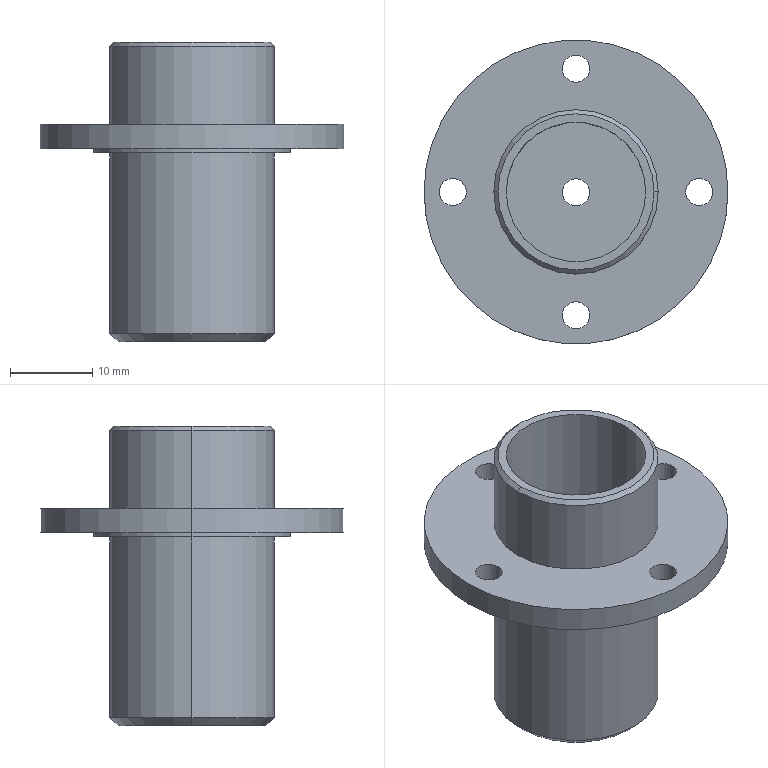Part | SolidWorks | features ICE 4, Chamfer 2, HoleWzd 2, 3DProfileFeature 1, Extrusion 1 | 1 solid | 30 faces | box 37 x 37 x 36.5 mm | volume 6267 mm3 | cylinder 20 | plane 6 | cone 4 | commonest cylinder face diameters 3.3 x10 20 x4 17 x2 24 x2 37 x2
STEP:
#1=CARTESIAN_POINT('',(9.5,0.,10.));
#2=VERTEX_POINT('',#1);
#3=CARTESIAN_POINT('',(-9.5,0.,10.));
#4=VERTEX_POINT('',#3);
#5=CARTESIAN_POINT('',(0.,0.,10.));
#6=DIRECTION('',(0.,0.,1.));
#7=DIRECTION('',(1.,0.,0.));
#8=AXIS2_PLACEMENT_3D('',#5,#6,#7);
#9=CIRCLE('',#8,9.5);
#10=EDGE_CURVE('',#2,#4,#9,.T.);
#11=ORIENTED_EDGE('',*,*,#10,.F.);
#12=CARTESIAN_POINT('',(10.,0.,9.5));
#13=VERTEX_POINT('',#12);
#14=CARTESIAN_POINT('',(9.5,0.,10.));
#15=DIRECTION('',(0.7071,0.,-0.7071));
#16=VECTOR('',#15,1000.);
#17=LINE('',#14,#16);
#18=EDGE_CURVE('',#2,#13,#17,.T.);
#19=ORIENTED_EDGE('',*,*,#18,.T.);
#20=CARTESIAN_POINT('',(-10.,0.,9.5));
#21=VERTEX_POINT('',#20);
#22=CARTESIAN_POINT('',(0.,0.,9.5));
#23=DIRECTION('',(0.,0.,-1.));
#24=DIRECTION('',(1.,0.,0.));
#25=AXIS2_PLACEMENT_3D('',#22,#23,#24);
#26=CIRCLE('',#25,10.);
#27=EDGE_CURVE('',#21,#13,#26,.T.);
#28=ORIENTED_EDGE('',*,*,#27,.F.);
#29=CARTESIAN_POINT('',(-9.5,0.,10.));
#30=DIRECTION('',(-0.7071,0.,-0.7071));
#31=VECTOR('',#30,1000.);
#32=LINE('',#29,#31);
#33=EDGE_CURVE('',#4,#21,#32,.T.);
#34=ORIENTED_EDGE('',*,*,#33,.F.);
#35=EDGE_LOOP('',(#11,#19,#28,#34));
#36=FACE_OUTER_BOUND('',#35,.T.);
#37=CARTESIAN_POINT('',(0.,0.,10.));
#38=DIRECTION('',(0.,0.,-1.));
#39=DIRECTION('',(-1.,0.,0.));
#40=AXIS2_PLACEMENT_3D('',#37,#38,#39);
#41=CONICAL_SURFACE('',#40,9.5,0.7854);
#42=ADVANCED_FACE('',(#36),#41,.T.);
#43=CARTESIAN_POINT('',(1.65,0.,-22.5));
#44=VERTEX_POINT('',#43);
#45=CARTESIAN_POINT('',(-1.65,0.,-22.5));
#46=VERTEX_POINT('',#45);
#47=CARTESIAN_POINT('',(0.,0.,-22.5));
#48=DIRECTION('',(0.,0.,-1.));
#49=DIRECTION('',(-1.,0.,0.));
#50=AXIS2_PLACEMENT_3D('',#47,#48,#49);
#51=CIRCLE('',#50,1.65);
#52=EDGE_CURVE('',#44,#46,#51,.T.);
#53=ORIENTED_EDGE('',*,*,#52,.F.);
#54=CARTESIAN_POINT('',(1.65,0.,-26.5));
#55=VERTEX_POINT('',#54);
#56=CARTESIAN_POINT('',(1.65,0.,-26.5));
#57=DIRECTION('',(0.,0.,-1.));
#58=VECTOR('',#57,1000.);
#59=LINE('',#56,#58);
#60=EDGE_CURVE('',#44,#55,#59,.T.);
#61=ORIENTED_EDGE('',*,*,#60,.T.);
#62=CARTESIAN_POINT('',(-1.65,0.,-26.5));
#63=VERTEX_POINT('',#62);
#64=CARTESIAN_POINT('',(0.,0.,-26.5));
#65=DIRECTION('',(0.,0.,-1.));
#66=DIRECTION('',(-1.,0.,0.));
#67=AXIS2_PLACEMENT_3D('',#64,#65,#66);
#68=CIRCLE('',#67,1.65);
#69=EDGE_CURVE('',#55,#63,#68,.T.);
#70=ORIENTED_EDGE('',*,*,#69,.T.);
#71=CARTESIAN_POINT('',(-1.65,0.,-26.5));
#72=DIRECTION('',(0.,0.,-1.));
#73=VECTOR('',#72,1000.);
#74=LINE('',#71,#73);
#75=EDGE_CURVE('',#46,#63,#74,.T.);
#76=ORIENTED_EDGE('',*,*,#75,.F.);
#77=EDGE_LOOP('',(#53,#61,#70,#76));
#78=FACE_OUTER_BOUND('',#77,.T.);
#79=CARTESIAN_POINT('',(0.,0.,-26.5));
#80=DIRECTION('',(0.,0.,-1.));
#81=DIRECTION('',(-1.,0.,0.));
#82=AXIS2_PLACEMENT_3D('',#79,#80,#81);
#83=CYLINDRICAL_SURFACE('',#82,1.65);
#84=ADVANCED_FACE('',(#78),#83,.F.);
#85=CARTESIAN_POINT('',(-9.,0.,-26.5));
#86=VERTEX_POINT('',#85);
#87=CARTESIAN_POINT('',(9.,0.,-26.5));
#88=VERTEX_POINT('',#87);
#89=CARTESIAN_POINT('',(0.,0.,-26.5));
#90=DIRECTION('',(0.,0.,-1.));
#91=DIRECTION('',(-1.,0.,0.));
#92=AXIS2_PLACEMENT_3D('',#89,#90,#91);
#93=CIRCLE('',#92,9.);
#94=EDGE_CURVE('',#86,#88,#93,.T.);
#95=ORIENTED_EDGE('',*,*,#94,.F.);
#96=CARTESIAN_POINT('',(-10.,0.,-25.5));
#97=VERTEX_POINT('',#96);
#98=CARTESIAN_POINT('',(-9.,0.,-26.5));
#99=DIRECTION('',(-0.7071,0.,0.7071));
#100=VECTOR('',#99,1000.);
#101=LINE('',#98,#100);
#102=EDGE_CURVE('',#86,#97,#101,.T.);
#103=ORIENTED_EDGE('',*,*,#102,.T.);
#104=CARTESIAN_POINT('',(10.,0.,-25.5));
#105=VERTEX_POINT('',#104);
#106=CARTESIAN_POINT('',(0.,0.,-25.5));
#107=DIRECTION('',(0.,0.,1.));
#108=DIRECTION('',(-1.,0.,0.));
#109=AXIS2_PLACEMENT_3D('',#106,#107,#108);
#110=CIRCLE('',#109,10.);
#111=EDGE_CURVE('',#105,#97,#110,.T.);
#112=ORIENTED_EDGE('',*,*,#111,.F.);
#113=CARTESIAN_POINT('',(9.,0.,-26.5));
#114=DIRECTION('',(0.7071,0.,0.7071));
#115=VECTOR('',#114,1000.);
#116=LINE('',#113,#115);
#117=EDGE_CURVE('',#88,#105,#116,.T.);
#118=ORIENTED_EDGE('',*,*,#117,.F.);
#119=EDGE_LOOP('',(#95,#103,#112,#118));
#120=FACE_OUTER_BOUND('',#119,.T.);
#121=CARTESIAN_POINT('',(0.,0.,-26.5));
#122=DIRECTION('',(0.,0.,1.));
#123=DIRECTION('',(1.,0.,0.));
#124=AXIS2_PLACEMENT_3D('',#121,#122,#123);
#125=CONICAL_SURFACE('',#124,9.,0.7854);
#126=ADVANCED_FACE('',(#120),#125,.T.);
#127=CARTESIAN_POINT('',(-13.35,0.,-3.));
#128=VERTEX_POINT('',#127);
#129=CARTESIAN_POINT('',(-16.65,0.,-3.));
#130=VERTEX_POINT('',#129);
#131=CARTESIAN_POINT('',(-15.,0.,-3.));
#132=DIRECTION('',(0.,0.,-1.));
#133=DIRECTION('',(-1.,0.,0.));
#134=AXIS2_PLACEMENT_3D('',#131,#132,#133);
#135=CIRCLE('',#134,1.65);
#136=EDGE_CURVE('',#128,#130,#135,.T.);
#137=ORIENTED_EDGE('',*,*,#136,.T.);
#138=CARTESIAN_POINT('',(-16.65,0.,0.));
#139=VERTEX_POINT('',#138);
#140=CARTESIAN_POINT('',(-16.65,0.,0.));
#141=DIRECTION('',(0.,0.,1.));
#142=VECTOR('',#141,1000.);
#143=LINE('',#140,#142);
#144=EDGE_CURVE('',#130,#139,#143,.T.);
#145=ORIENTED_EDGE('',*,*,#144,.T.);
#146=CARTESIAN_POINT('',(-13.35,0.,0.));
#147=VERTEX_POINT('',#146);
#148=CARTESIAN_POINT('',(-15.,0.,0.));
#149=DIRECTION('',(0.,0.,1.));
#150=DIRECTION('',(1.,0.,0.));
#151=AXIS2_PLACEMENT_3D('',#148,#149,#150);
#152=CIRCLE('',#151,1.65);
#153=EDGE_CURVE('',#139,#147,#152,.T.);
#154=ORIENTED_EDGE('',*,*,#153,.T.);
#155=CARTESIAN_POINT('',(-13.35,0.,0.));
#156=DIRECTION('',(0.,0.,1.));
#157=VECTOR('',#156,1000.);
#158=LINE('',#155,#157);
#159=EDGE_CURVE('',#128,#147,#158,.T.);
#160=ORIENTED_EDGE('',*,*,#159,.F.);
#161=EDGE_LOOP('',(#137,#145,#154,#160));
#162=FACE_OUTER_BOUND('',#161,.T.);
#163=CARTESIAN_POINT('',(-15.,0.,0.));
#164=DIRECTION('',(0.,0.,1.));
#165=DIRECTION('',(1.,0.,0.));
#166=AXIS2_PLACEMENT_3D('',#163,#164,#165);
#167=CYLINDRICAL_SURFACE('',#166,1.65);
#168=ADVANCED_FACE('',(#162),#167,.F.);
#169=CARTESIAN_POINT('',(1.65,15.,-3.));
#170=VERTEX_POINT('',#169);
#171=CARTESIAN_POINT('',(-1.65,15.,-3.));
#172=VERTEX_POINT('',#171);
#173=CARTESIAN_POINT('',(0.,15.,-3.));
#174=DIRECTION('',(0.,0.,-1.));
#175=DIRECTION('',(-1.,0.,0.));
#176=AXIS2_PLACEMENT_3D('',#173,#174,#175);
#177=CIRCLE('',#176,1.65);
#178=EDGE_CURVE('',#170,#172,#177,.T.);
#179=ORIENTED_EDGE('',*,*,#178,.T.);
#180=CARTESIAN_POINT('',(-1.65,15.,0.));
#181=VERTEX_POINT('',#180);
#182=CARTESIAN_POINT('',(-1.65,15.,0.));
#183=DIRECTION('',(0.,0.,1.));
#184=VECTOR('',#183,1000.);
#185=LINE('',#182,#184);
#186=EDGE_CURVE('',#172,#181,#185,.T.);
#187=ORIENTED_EDGE('',*,*,#186,.T.);
#188=CARTESIAN_POINT('',(1.65,15.,0.));
#189=VERTEX_POINT('',#188);
#190=CARTESIAN_POINT('',(0.,15.,0.));
#191=DIRECTION('',(0.,0.,1.));
#192=DIRECTION('',(1.,0.,0.));
#193=AXIS2_PLACEMENT_3D('',#190,#191,#192);
#194=CIRCLE('',#193,1.65);
#195=EDGE_CURVE('',#181,#189,#194,.T.);
#196=ORIENTED_EDGE('',*,*,#195,.T.);
#197=CARTESIAN_POINT('',(1.65,15.,0.));
#198=DIRECTION('',(0.,0.,1.));
#199=VECTOR('',#198,1000.);
#200=LINE('',#197,#199);
#201=EDGE_CURVE('',#170,#189,#200,.T.);
#202=ORIENTED_EDGE('',*,*,#201,.F.);
#203=EDGE_LOOP('',(#179,#187,#196,#202));
#204=FACE_OUTER_BOUND('',#203,.T.);
#205=CARTESIAN_POINT('',(0.,15.,0.));
#206=DIRECTION('',(0.,0.,1.));
#207=DIRECTION('',(1.,0.,0.));
#208=AXIS2_PLACEMENT_3D('',#205,#206,#207);
#209=CYLINDRICAL_SURFACE('',#208,1.65);
#210=ADVANCED_FACE('',(#204),#209,.F.);
#211=CARTESIAN_POINT('',(16.65,0.,-3.));
#212=VERTEX_POINT('',#211);
#213=CARTESIAN_POINT('',(13.35,0.,-3.));
#214=VERTEX_POINT('',#213);
#215=CARTESIAN_POINT('',(15.,0.,-3.));
#216=DIRECTION('',(0.,0.,-1.));
#217=DIRECTION('',(-1.,0.,0.));
#218=AXIS2_PLACEMENT_3D('',#215,#216,#217);
#219=CIRCLE('',#218,1.65);
#220=EDGE_CURVE('',#212,#214,#219,.T.);
#221=ORIENTED_EDGE('',*,*,#220,.T.);
#222=CARTESIAN_POINT('',(13.35,0.,0.));
#223=VERTEX_POINT('',#222);
#224=CARTESIAN_POINT('',(13.35,0.,0.));
#225=DIRECTION('',(0.,0.,1.));
#226=VECTOR('',#225,1000.);
#227=LINE('',#224,#226);
#228=EDGE_CURVE('',#214,#223,#227,.T.);
#229=ORIENTED_EDGE('',*,*,#228,.T.);
#230=CARTESIAN_POINT('',(16.65,0.,0.));
#231=VERTEX_POINT('',#230);
#232=CARTESIAN_POINT('',(15.,0.,0.));
#233=DIRECTION('',(0.,0.,1.));
#234=DIRECTION('',(1.,0.,0.));
#235=AXIS2_PLACEMENT_3D('',#232,#233,#234);
#236=CIRCLE('',#235,1.65);
#237=EDGE_CURVE('',#223,#231,#236,.T.);
#238=ORIENTED_EDGE('',*,*,#237,.T.);
#239=CARTESIAN_POINT('',(16.65,0.,0.));
#240=DIRECTION('',(0.,0.,1.));
#241=VECTOR('',#240,1000.);
#242=LINE('',#239,#241);
#243=EDGE_CURVE('',#212,#231,#242,.T.);
#244=ORIENTED_EDGE('',*,*,#243,.F.);
#245=EDGE_LOOP('',(#221,#229,#238,#244));
#246=FACE_OUTER_BOUND('',#245,.T.);
#247=CARTESIAN_POINT('',(15.,0.,0.));
#248=DIRECTION('',(0.,0.,1.));
#249=DIRECTION('',(1.,0.,0.));
#250=AXIS2_PLACEMENT_3D('',#247,#248,#249);
#251=CYLINDRICAL_SURFACE('',#250,1.65);
#252=ADVANCED_FACE('',(#246),#251,.F.);
#253=CARTESIAN_POINT('',(1.65,-15.,-3.));
#254=VERTEX_POINT('',#253);
#255=CARTESIAN_POINT('',(-1.65,-15.,-3.));
#256=VERTEX_POINT('',#255);
#257=CARTESIAN_POINT('',(0.,-15.,-3.));
#258=DIRECTION('',(0.,0.,-1.));
#259=DIRECTION('',(-1.,0.,0.));
#260=AXIS2_PLACEMENT_3D('',#257,#258,#259);
#261=CIRCLE('',#260,1.65);
#262=EDGE_CURVE('',#254,#256,#261,.T.);
#263=ORIENTED_EDGE('',*,*,#262,.T.);
#264=CARTESIAN_POINT('',(-1.65,-15.,0.));
#265=VERTEX_POINT('',#264);
#266=CARTESIAN_POINT('',(-1.65,-15.,0.));
#267=DIRECTION('',(0.,0.,1.));
#268=VECTOR('',#267,1000.);
#269=LINE('',#266,#268);
#270=EDGE_CURVE('',#256,#265,#269,.T.);
#271=ORIENTED_EDGE('',*,*,#270,.T.);
#272=CARTESIAN_POINT('',(1.65,-15.,0.));
#273=VERTEX_POINT('',#272);
#274=CARTESIAN_POINT('',(0.,-15.,0.));
#275=DIRECTION('',(0.,0.,1.));
#276=DIRECTION('',(1.,0.,0.));
#277=AXIS2_PLACEMENT_3D('',#274,#275,#276);
#278=CIRCLE('',#277,1.65);
#279=EDGE_CURVE('',#265,#273,#278,.T.);
#280=ORIENTED_EDGE('',*,*,#279,.T.);
#281=CARTESIAN_POINT('',(1.65,-15.,0.));
#282=DIRECTION('',(0.,0.,1.));
#283=VECTOR('',#282,1000.);
#284=LINE('',#281,#283);
#285=EDGE_CURVE('',#254,#273,#284,.T.);
#286=ORIENTED_EDGE('',*,*,#285,.F.);
#287=EDGE_LOOP('',(#263,#271,#280,#286));
#288=FACE_OUTER_BOUND('',#287,.T.);
#289=CARTESIAN_POINT('',(0.,-15.,0.));
#290=DIRECTION('',(0.,0.,1.));
#291=DIRECTION('',(1.,0.,0.));
#292=AXIS2_PLACEMENT_3D('',#289,#290,#291);
#293=CYLINDRICAL_SURFACE('',#292,1.65);
#294=ADVANCED_FACE('',(#288),#293,.F.);
#295=CARTESIAN_POINT('',(-12.,0.,-3.5));
#296=VERTEX_POINT('',#295);
#297=CARTESIAN_POINT('',(12.,0.,-3.5));
#298=VERTEX_POINT('',#297);
#299=CARTESIAN_POINT('',(0.,0.,-3.5));
#300=DIRECTION('',(0.,0.,-1.));
#301=DIRECTION('',(-1.,0.,0.));
#302=AXIS2_PLACEMENT_3D('',#299,#300,#301);
#303=CIRCLE('',#302,12.);
#304=EDGE_CURVE('',#296,#298,#303,.T.);
#305=ORIENTED_EDGE('',*,*,#304,.F.);
#306=CARTESIAN_POINT('',(-12.,0.,-3.));
#307=VERTEX_POINT('',#306);
#308=CARTESIAN_POINT('',(-12.,0.,-3.5));
#309=DIRECTION('',(0.,0.,1.));
#310=VECTOR('',#309,1000.);
#311=LINE('',#308,#310);
#312=EDGE_CURVE('',#296,#307,#311,.T.);
#313=ORIENTED_EDGE('',*,*,#312,.T.);
#314=CARTESIAN_POINT('',(12.,0.,-3.));
#315=VERTEX_POINT('',#314);
#316=CARTESIAN_POINT('',(0.,0.,-3.));
#317=DIRECTION('',(0.,0.,-1.));
#318=DIRECTION('',(-1.,0.,0.));
#319=AXIS2_PLACEMENT_3D('',#316,#317,#318);
#320=CIRCLE('',#319,12.);
#321=EDGE_CURVE('',#307,#315,#320,.T.);
#322=ORIENTED_EDGE('',*,*,#321,.T.);
#323=CARTESIAN_POINT('',(12.,0.,-3.5));
#324=DIRECTION('',(0.,0.,1.));
#325=VECTOR('',#324,1000.);
#326=LINE('',#323,#325);
#327=EDGE_CURVE('',#298,#315,#326,.T.);
#328=ORIENTED_EDGE('',*,*,#327,.F.);
#329=EDGE_LOOP('',(#305,#313,#322,#328));
#330=FACE_OUTER_BOUND('',#329,.T.);
#331=CARTESIAN_POINT('',(0.,0.,-3.5));
#332=DIRECTION('',(0.,0.,1.));
#333=DIRECTION('',(1.,0.,0.));
#334=AXIS2_PLACEMENT_3D('',#331,#332,#333);
#335=CYLINDRICAL_SURFACE('',#334,12.);
#336=ADVANCED_FACE('',(#330),#335,.T.);
#337=ORIENTED_EDGE('',*,*,#111,.T.);
#338=CARTESIAN_POINT('',(-10.,0.,-3.5));
#339=VERTEX_POINT('',#338);
#340=CARTESIAN_POINT('',(-10.,0.,-26.5));
#341=DIRECTION('',(0.,0.,1.));
#342=VECTOR('',#341,1000.);
#343=LINE('',#340,#342);
#344=EDGE_CURVE('',#97,#339,#343,.T.);
#345=ORIENTED_EDGE('',*,*,#344,.T.);
#346=CARTESIAN_POINT('',(10.,0.,-3.5));
#347=VERTEX_POINT('',#346);
#348=CARTESIAN_POINT('',(0.,0.,-3.5));
#349=DIRECTION('',(0.,0.,-1.));
#350=DIRECTION('',(-1.,0.,0.));
#351=AXIS2_PLACEMENT_3D('',#348,#349,#350);
#352=CIRCLE('',#351,10.);
#353=EDGE_CURVE('',#339,#347,#352,.T.);
#354=ORIENTED_EDGE('',*,*,#353,.T.);
#355=CARTESIAN_POINT('',(10.,0.,-26.5));
#356=DIRECTION('',(0.,0.,1.));
#357=VECTOR('',#356,1000.);
#358=LINE('',#355,#357);
#359=EDGE_CURVE('',#105,#347,#358,.T.);
#360=ORIENTED_EDGE('',*,*,#359,.F.);
#361=EDGE_LOOP('',(#337,#345,#354,#360));
#362=FACE_OUTER_BOUND('',#361,.T.);
#363=CARTESIAN_POINT('',(0.,0.,-26.5));
#364=DIRECTION('',(0.,0.,1.));
#365=DIRECTION('',(1.,0.,0.));
#366=AXIS2_PLACEMENT_3D('',#363,#364,#365);
#367=CYLINDRICAL_SURFACE('',#366,10.);
#368=ADVANCED_FACE('',(#362),#367,.T.);
#369=CARTESIAN_POINT('',(-18.5,0.,-3.));
#370=VERTEX_POINT('',#369);
#371=CARTESIAN_POINT('',(18.5,0.,-3.));
#372=VERTEX_POINT('',#371);
#373=CARTESIAN_POINT('',(0.,0.,-3.));
#374=DIRECTION('',(0.,0.,-1.));
#375=DIRECTION('',(-1.,0.,0.));
#376=AXIS2_PLACEMENT_3D('',#373,#374,#375);
#377=CIRCLE('',#376,18.5);
#378=EDGE_CURVE('',#370,#372,#377,.T.);
#379=ORIENTED_EDGE('',*,*,#378,.F.);
#380=CARTESIAN_POINT('',(-18.5,0.,0.));
#381=VERTEX_POINT('',#380);
#382=CARTESIAN_POINT('',(-18.5,0.,-3.));
#383=DIRECTION('',(0.,0.,1.));
#384=VECTOR('',#383,1000.);
#385=LINE('',#382,#384);
#386=EDGE_CURVE('',#370,#381,#385,.T.);
#387=ORIENTED_EDGE('',*,*,#386,.T.);
#388=CARTESIAN_POINT('',(18.5,0.,0.));
#389=VERTEX_POINT('',#388);
#390=CARTESIAN_POINT('',(0.,0.,0.));
#391=DIRECTION('',(0.,0.,-1.));
#392=DIRECTION('',(-1.,0.,0.));
#393=AXIS2_PLACEMENT_3D('',#390,#391,#392);
#394=CIRCLE('',#393,18.5);
#395=EDGE_CURVE('',#381,#389,#394,.T.);
#396=ORIENTED_EDGE('',*,*,#395,.T.);
#397=CARTESIAN_POINT('',(18.5,0.,-3.));
#398=DIRECTION('',(0.,0.,1.));
#399=VECTOR('',#398,1000.);
#400=LINE('',#397,#399);
#401=EDGE_CURVE('',#372,#389,#400,.T.);
#402=ORIENTED_EDGE('',*,*,#401,.F.);
#403=EDGE_LOOP('',(#379,#387,#396,#402));
#404=FACE_OUTER_BOUND('',#403,.T.);
#405=CARTESIAN_POINT('',(0.,0.,-3.));
#406=DIRECTION('',(0.,0.,1.));
#407=DIRECTION('',(1.,0.,0.));
#408=AXIS2_PLACEMENT_3D('',#405,#406,#407);
#409=CYLINDRICAL_SURFACE('',#408,18.5);
#410=ADVANCED_FACE('',(#404),#409,.T.);
#411=ORIENTED_EDGE('',*,*,#27,.T.);
#412=CARTESIAN_POINT('',(10.,0.,0.));
#413=VERTEX_POINT('',#412);
#414=CARTESIAN_POINT('',(10.,0.,10.));
#415=DIRECTION('',(0.,0.,-1.));
#416=VECTOR('',#415,1000.);
#417=LINE('',#414,#416);
#418=EDGE_CURVE('',#13,#413,#417,.T.);
#419=ORIENTED_EDGE('',*,*,#418,.T.);
#420=CARTESIAN_POINT('',(-10.,0.,0.));
#421=VERTEX_POINT('',#420);
#422=CARTESIAN_POINT('',(0.,0.,0.));
#423=DIRECTION('',(0.,0.,1.));
#424=DIRECTION('',(1.,0.,0.));
#425=AXIS2_PLACEMENT_3D('',#422,#423,#424);
#426=CIRCLE('',#425,10.);
#427=EDGE_CURVE('',#413,#421,#426,.T.);
#428=ORIENTED_EDGE('',*,*,#427,.T.);
#429=CARTESIAN_POINT('',(-10.,0.,10.));
#430=DIRECTION('',(0.,0.,-1.));
#431=VECTOR('',#430,1000.);
#432=LINE('',#429,#431);
#433=EDGE_CURVE('',#21,#421,#432,.T.);
#434=ORIENTED_EDGE('',*,*,#433,.F.);
#435=EDGE_LOOP('',(#411,#419,#428,#434));
#436=FACE_OUTER_BOUND('',#435,.T.);
#437=CARTESIAN_POINT('',(0.,0.,10.));
#438=DIRECTION('',(0.,0.,-1.));
#439=DIRECTION('',(-1.,0.,0.));
#440=AXIS2_PLACEMENT_3D('',#437,#438,#439);
#441=CYLINDRICAL_SURFACE('',#440,10.);
#442=ADVANCED_FACE('',(#436),#441,.T.);
#443=CARTESIAN_POINT('',(-8.5,0.,10.));
#444=VERTEX_POINT('',#443);
#445=CARTESIAN_POINT('',(8.5,0.,10.));
#446=VERTEX_POINT('',#445);
#447=CARTESIAN_POINT('',(0.,0.,10.));
#448=DIRECTION('',(0.,0.,1.));
#449=DIRECTION('',(1.,0.,0.));
#450=AXIS2_PLACEMENT_3D('',#447,#448,#449);
#451=CIRCLE('',#450,8.5);
#452=EDGE_CURVE('',#444,#446,#451,.T.);
#453=ORIENTED_EDGE('',*,*,#452,.T.);
#454=CARTESIAN_POINT('',(8.5,0.,-22.5));
#455=VERTEX_POINT('',#454);
#456=CARTESIAN_POINT('',(8.5,0.,10.));
#457=DIRECTION('',(0.,0.,-1.));
#458=VECTOR('',#457,1000.);
#459=LINE('',#456,#458);
#460=EDGE_CURVE('',#446,#455,#459,.T.);
#461=ORIENTED_EDGE('',*,*,#460,.T.);
#462=CARTESIAN_POINT('',(-8.5,0.,-22.5));
#463=VERTEX_POINT('',#462);
#464=CARTESIAN_POINT('',(0.,0.,-22.5));
#465=DIRECTION('',(0.,0.,-1.));
#466=DIRECTION('',(-1.,0.,0.));
#467=AXIS2_PLACEMENT_3D('',#464,#465,#466);
#468=CIRCLE('',#467,8.5);
#469=EDGE_CURVE('',#455,#463,#468,.T.);
#470=ORIENTED_EDGE('',*,*,#469,.T.);
#471=CARTESIAN_POINT('',(-8.5,0.,10.));
#472=DIRECTION('',(0.,0.,-1.));
#473=VECTOR('',#472,1000.);
#474=LINE('',#471,#473);
#475=EDGE_CURVE('',#444,#463,#474,.T.);
#476=ORIENTED_EDGE('',*,*,#475,.F.);
#477=EDGE_LOOP('',(#453,#461,#470,#476));
#478=FACE_OUTER_BOUND('',#477,.T.);
#479=CARTESIAN_POINT('',(0.,0.,10.));
#480=DIRECTION('',(0.,0.,-1.));
#481=DIRECTION('',(-1.,0.,0.));
#482=AXIS2_PLACEMENT_3D('',#479,#480,#481);
#483=CYLINDRICAL_SURFACE('',#482,8.5);
#484=ADVANCED_FACE('',(#478),#483,.F.);
#485=ORIENTED_EDGE('',*,*,#460,.F.);
#486=CARTESIAN_POINT('',(0.,0.,10.));
#487=DIRECTION('',(0.,0.,1.));
#488=DIRECTION('',(1.,0.,0.));
#489=AXIS2_PLACEMENT_3D('',#486,#487,#488);
#490=CIRCLE('',#489,8.5);
#491=EDGE_CURVE('',#446,#444,#490,.T.);
#492=ORIENTED_EDGE('',*,*,#491,.T.);
#493=ORIENTED_EDGE('',*,*,#475,.T.);
#494=CARTESIAN_POINT('',(0.,0.,-22.5));
#495=DIRECTION('',(0.,0.,-1.));
#496=DIRECTION('',(-1.,0.,0.));
#497=AXIS2_PLACEMENT_3D('',#494,#495,#496);
#498=CIRCLE('',#497,8.5);
#499=EDGE_CURVE('',#463,#455,#498,.T.);
#500=ORIENTED_EDGE('',*,*,#499,.T.);
#501=EDGE_LOOP('',(#485,#492,#493,#500));
#502=FACE_OUTER_BOUND('',#501,.T.);
#503=CARTESIAN_POINT('',(0.,0.,10.));
#504=DIRECTION('',(0.,0.,-1.));
#505=DIRECTION('',(-1.,0.,0.));
#506=AXIS2_PLACEMENT_3D('',#503,#504,#505);
#507=CYLINDRICAL_SURFACE('',#506,8.5);
#508=ADVANCED_FACE('',(#502),#507,.F.);
#509=ORIENTED_EDGE('',*,*,#136,.F.);
#510=CARTESIAN_POINT('',(-15.,0.,-3.));
#511=DIRECTION('',(0.,0.,-1.));
#512=DIRECTION('',(-1.,0.,0.));
#513=AXIS2_PLACEMENT_3D('',#510,#511,#512);
#514=CIRCLE('',#513,1.65);
#515=EDGE_CURVE('',#130,#128,#514,.T.);
#516=ORIENTED_EDGE('',*,*,#515,.F.);
#517=EDGE_LOOP('',(#509,#516));
#518=FACE_BOUND('',#517,.T.);
#519=ORIENTED_EDGE('',*,*,#178,.F.);
#520=CARTESIAN_POINT('',(0.,15.,-3.));
#521=DIRECTION('',(0.,0.,-1.));
#522=DIRECTION('',(-1.,0.,0.));
#523=AXIS2_PLACEMENT_3D('',#520,#521,#522);
#524=CIRCLE('',#523,1.65);
#525=EDGE_CURVE('',#172,#170,#524,.T.);
#526=ORIENTED_EDGE('',*,*,#525,.F.);
#527=EDGE_LOOP('',(#519,#526));
#528=FACE_BOUND('',#527,.T.);
#529=ORIENTED_EDGE('',*,*,#220,.F.);
#530=CARTESIAN_POINT('',(15.,0.,-3.));
#531=DIRECTION('',(0.,0.,-1.));
#532=DIRECTION('',(-1.,0.,0.));
#533=AXIS2_PLACEMENT_3D('',#530,#531,#532);
#534=CIRCLE('',#533,1.65);
#535=EDGE_CURVE('',#214,#212,#534,.T.);
#536=ORIENTED_EDGE('',*,*,#535,.F.);
#537=EDGE_LOOP('',(#529,#536));
#538=FACE_BOUND('',#537,.T.);
#539=ORIENTED_EDGE('',*,*,#262,.F.);
#540=CARTESIAN_POINT('',(0.,-15.,-3.));
#541=DIRECTION('',(0.,0.,-1.));
#542=DIRECTION('',(-1.,0.,0.));
#543=AXIS2_PLACEMENT_3D('',#540,#541,#542);
#544=CIRCLE('',#543,1.65);
#545=EDGE_CURVE('',#256,#254,#544,.T.);
#546=ORIENTED_EDGE('',*,*,#545,.F.);
#547=EDGE_LOOP('',(#539,#546));
#548=FACE_BOUND('',#547,.T.);
#549=CARTESIAN_POINT('',(0.,0.,-3.));
#550=DIRECTION('',(0.,0.,-1.));
#551=DIRECTION('',(-1.,0.,0.));
#552=AXIS2_PLACEMENT_3D('',#549,#550,#551);
#553=CIRCLE('',#552,18.5);
#554=EDGE_CURVE('',#372,#370,#553,.T.);
#555=ORIENTED_EDGE('',*,*,#554,.T.);
#556=ORIENTED_EDGE('',*,*,#378,.T.);
#557=EDGE_LOOP('',(#555,#556));
#558=FACE_OUTER_BOUND('',#557,.T.);
#559=CARTESIAN_POINT('',(0.,0.,-3.));
#560=DIRECTION('',(0.,0.,-1.));
#561=DIRECTION('',(-1.,0.,0.));
#562=AXIS2_PLACEMENT_3D('',#559,#560,#561);
#563=CIRCLE('',#562,12.);
#564=EDGE_CURVE('',#315,#307,#563,.T.);
#565=ORIENTED_EDGE('',*,*,#564,.F.);
#566=ORIENTED_EDGE('',*,*,#321,.F.);
#567=EDGE_LOOP('',(#565,#566));
#568=FACE_BOUND('',#567,.T.);
#569=CARTESIAN_POINT('',(0.,0.,-3.));
#570=DIRECTION('',(0.,0.,-1.));
#571=DIRECTION('',(-1.,0.,0.));
#572=AXIS2_PLACEMENT_3D('',#569,#570,#571);
#573=PLANE('',#572);
#574=ADVANCED_FACE('',(#518,#528,#538,#548,#558,#568),#573,.T.);
#575=CARTESIAN_POINT('',(0.,0.,10.));
#576=DIRECTION('',(0.,0.,1.));
#577=DIRECTION('',(1.,0.,0.));
#578=AXIS2_PLACEMENT_3D('',#575,#576,#577);
#579=CIRCLE('',#578,9.5);
#580=EDGE_CURVE('',#4,#2,#579,.T.);
#581=ORIENTED_EDGE('',*,*,#580,.T.);
#582=ORIENTED_EDGE('',*,*,#10,.T.);
#583=EDGE_LOOP('',(#581,#582));
#584=FACE_OUTER_BOUND('',#583,.T.);
#585=ORIENTED_EDGE('',*,*,#452,.F.);
#586=ORIENTED_EDGE('',*,*,#491,.F.);
#587=EDGE_LOOP('',(#585,#586));
#588=FACE_BOUND('',#587,.T.);
#589=CARTESIAN_POINT('',(0.,0.,10.));
#590=DIRECTION('',(0.,0.,1.));
#591=DIRECTION('',(1.,0.,0.));
#592=AXIS2_PLACEMENT_3D('',#589,#590,#591);
#593=PLANE('',#592);
#594=ADVANCED_FACE('',(#584,#588),#593,.T.);
#595=ORIENTED_EDGE('',*,*,#418,.F.);
#596=CARTESIAN_POINT('',(0.,0.,9.5));
#597=DIRECTION('',(0.,0.,-1.));
#598=DIRECTION('',(1.,0.,0.));
#599=AXIS2_PLACEMENT_3D('',#596,#597,#598);
#600=CIRCLE('',#599,10.);
#601=EDGE_CURVE('',#13,#21,#600,.T.);
#602=ORIENTED_EDGE('',*,*,#601,.T.);
#603=ORIENTED_EDGE('',*,*,#433,.T.);
#604=CARTESIAN_POINT('',(0.,0.,0.));
#605=DIRECTION('',(0.,0.,1.));
#606=DIRECTION('',(1.,0.,0.));
#607=AXIS2_PLACEMENT_3D('',#604,#605,#606);
#608=CIRCLE('',#607,10.);
#609=EDGE_CURVE('',#421,#413,#608,.T.);
#610=ORIENTED_EDGE('',*,*,#609,.T.);
#611=EDGE_LOOP('',(#595,#602,#603,#610));
#612=FACE_OUTER_BOUND('',#611,.T.);
#613=CARTESIAN_POINT('',(0.,0.,10.));
#614=DIRECTION('',(0.,0.,-1.));
#615=DIRECTION('',(-1.,0.,0.));
#616=AXIS2_PLACEMENT_3D('',#613,#614,#615);
#617=CYLINDRICAL_SURFACE('',#616,10.);
#618=ADVANCED_FACE('',(#612),#617,.T.);
#619=CARTESIAN_POINT('',(-15.,0.,0.));
#620=DIRECTION('',(0.,0.,1.));
#621=DIRECTION('',(1.,0.,0.));
#622=AXIS2_PLACEMENT_3D('',#619,#620,#621);
#623=CIRCLE('',#622,1.65);
#624=EDGE_CURVE('',#147,#139,#623,.T.);
#625=ORIENTED_EDGE('',*,*,#624,.F.);
#626=ORIENTED_EDGE('',*,*,#153,.F.);
#627=EDGE_LOOP('',(#625,#626));
#628=FACE_BOUND('',#627,.T.);
#629=CARTESIAN_POINT('',(0.,15.,0.));
#630=DIRECTION('',(0.,0.,1.));
#631=DIRECTION('',(1.,0.,0.));
#632=AXIS2_PLACEMENT_3D('',#629,#630,#631);
#633=CIRCLE('',#632,1.65);
#634=EDGE_CURVE('',#189,#181,#633,.T.);
#635=ORIENTED_EDGE('',*,*,#634,.F.);
#636=ORIENTED_EDGE('',*,*,#195,.F.);
#637=EDGE_LOOP('',(#635,#636));
#638=FACE_BOUND('',#637,.T.);
#639=CARTESIAN_POINT('',(15.,0.,0.));
#640=DIRECTION('',(0.,0.,1.));
#641=DIRECTION('',(1.,0.,0.));
#642=AXIS2_PLACEMENT_3D('',#639,#640,#641);
#643=CIRCLE('',#642,1.65);
#644=EDGE_CURVE('',#231,#223,#643,.T.);
#645=ORIENTED_EDGE('',*,*,#644,.F.);
#646=ORIENTED_EDGE('',*,*,#237,.F.);
#647=EDGE_LOOP('',(#645,#646));
#648=FACE_BOUND('',#647,.T.);
#649=CARTESIAN_POINT('',(0.,-15.,0.));
#650=DIRECTION('',(0.,0.,1.));
#651=DIRECTION('',(1.,0.,0.));
#652=AXIS2_PLACEMENT_3D('',#649,#650,#651);
#653=CIRCLE('',#652,1.65);
#654=EDGE_CURVE('',#273,#265,#653,.T.);
#655=ORIENTED_EDGE('',*,*,#654,.F.);
#656=ORIENTED_EDGE('',*,*,#279,.F.);
#657=EDGE_LOOP('',(#655,#656));
#658=FACE_BOUND('',#657,.T.);
#659=ORIENTED_EDGE('',*,*,#609,.F.);
#660=ORIENTED_EDGE('',*,*,#427,.F.);
#661=EDGE_LOOP('',(#659,#660));
#662=FACE_BOUND('',#661,.T.);
#663=CARTESIAN_POINT('',(0.,0.,0.));
#664=DIRECTION('',(0.,0.,-1.));
#665=DIRECTION('',(-1.,0.,0.));
#666=AXIS2_PLACEMENT_3D('',#663,#664,#665);
#667=CIRCLE('',#666,18.5);
#668=EDGE_CURVE('',#389,#381,#667,.T.);
#669=ORIENTED_EDGE('',*,*,#668,.F.);
#670=ORIENTED_EDGE('',*,*,#395,.F.);
#671=EDGE_LOOP('',(#669,#670));
#672=FACE_OUTER_BOUND('',#671,.T.);
#673=CARTESIAN_POINT('',(0.,0.,0.));
#674=DIRECTION('',(0.,0.,-1.));
#675=DIRECTION('',(-1.,0.,0.));
#676=AXIS2_PLACEMENT_3D('',#673,#674,#675);
#677=PLANE('',#676);
#678=ADVANCED_FACE('',(#628,#638,#648,#658,#662,#672),#677,.F.);
#679=ORIENTED_EDGE('',*,*,#386,.F.);
#680=ORIENTED_EDGE('',*,*,#554,.F.);
#681=ORIENTED_EDGE('',*,*,#401,.T.);
#682=ORIENTED_EDGE('',*,*,#668,.T.);
#683=EDGE_LOOP('',(#679,#680,#681,#682));
#684=FACE_OUTER_BOUND('',#683,.T.);
#685=CARTESIAN_POINT('',(0.,0.,-3.));
#686=DIRECTION('',(0.,0.,1.));
#687=DIRECTION('',(1.,0.,0.));
#688=AXIS2_PLACEMENT_3D('',#685,#686,#687);
#689=CYLINDRICAL_SURFACE('',#688,18.5);
#690=ADVANCED_FACE('',(#684),#689,.T.);
#691=CARTESIAN_POINT('',(0.,0.,-26.5));
#692=DIRECTION('',(0.,0.,-1.));
#693=DIRECTION('',(-1.,0.,0.));
#694=AXIS2_PLACEMENT_3D('',#691,#692,#693);
#695=CIRCLE('',#694,1.65);
#696=EDGE_CURVE('',#63,#55,#695,.T.);
#697=ORIENTED_EDGE('',*,*,#696,.F.);
#698=ORIENTED_EDGE('',*,*,#69,.F.);
#699=EDGE_LOOP('',(#697,#698));
#700=FACE_BOUND('',#699,.T.);
#701=CARTESIAN_POINT('',(0.,0.,-26.5));
#702=DIRECTION('',(0.,0.,-1.));
#703=DIRECTION('',(-1.,0.,0.));
#704=AXIS2_PLACEMENT_3D('',#701,#702,#703);
#705=CIRCLE('',#704,9.);
#706=EDGE_CURVE('',#88,#86,#705,.T.);
#707=ORIENTED_EDGE('',*,*,#706,.T.);
#708=ORIENTED_EDGE('',*,*,#94,.T.);
#709=EDGE_LOOP('',(#707,#708));
#710=FACE_OUTER_BOUND('',#709,.T.);
#711=CARTESIAN_POINT('',(0.,0.,-26.5));
#712=DIRECTION('',(0.,0.,-1.));
#713=DIRECTION('',(-1.,0.,0.));
#714=AXIS2_PLACEMENT_3D('',#711,#712,#713);
#715=PLANE('',#714);
#716=ADVANCED_FACE('',(#700,#710),#715,.T.);
#717=ORIENTED_EDGE('',*,*,#344,.F.);
#718=CARTESIAN_POINT('',(0.,0.,-25.5));
#719=DIRECTION('',(0.,0.,1.));
#720=DIRECTION('',(-1.,0.,0.));
#721=AXIS2_PLACEMENT_3D('',#718,#719,#720);
#722=CIRCLE('',#721,10.);
#723=EDGE_CURVE('',#97,#105,#722,.T.);
#724=ORIENTED_EDGE('',*,*,#723,.T.);
#725=ORIENTED_EDGE('',*,*,#359,.T.);
#726=CARTESIAN_POINT('',(0.,0.,-3.5));
#727=DIRECTION('',(0.,0.,-1.));
#728=DIRECTION('',(-1.,0.,0.));
#729=AXIS2_PLACEMENT_3D('',#726,#727,#728);
#730=CIRCLE('',#729,10.);
#731=EDGE_CURVE('',#347,#339,#730,.T.);
#732=ORIENTED_EDGE('',*,*,#731,.T.);
#733=EDGE_LOOP('',(#717,#724,#725,#732));
#734=FACE_OUTER_BOUND('',#733,.T.);
#735=CARTESIAN_POINT('',(0.,0.,-26.5));
#736=DIRECTION('',(0.,0.,1.));
#737=DIRECTION('',(1.,0.,0.));
#738=AXIS2_PLACEMENT_3D('',#735,#736,#737);
#739=CYLINDRICAL_SURFACE('',#738,10.);
#740=ADVANCED_FACE('',(#734),#739,.T.);
#741=CARTESIAN_POINT('',(0.,0.,-3.5));
#742=DIRECTION('',(0.,0.,-1.));
#743=DIRECTION('',(-1.,0.,0.));
#744=AXIS2_PLACEMENT_3D('',#741,#742,#743);
#745=CIRCLE('',#744,12.);
#746=EDGE_CURVE('',#298,#296,#745,.T.);
#747=ORIENTED_EDGE('',*,*,#746,.T.);
#748=ORIENTED_EDGE('',*,*,#304,.T.);
#749=EDGE_LOOP('',(#747,#748));
#750=FACE_OUTER_BOUND('',#749,.T.);
#751=ORIENTED_EDGE('',*,*,#731,.F.);
#752=ORIENTED_EDGE('',*,*,#353,.F.);
#753=EDGE_LOOP('',(#751,#752));
#754=FACE_BOUND('',#753,.T.);
#755=CARTESIAN_POINT('',(0.,0.,-3.5));
#756=DIRECTION('',(0.,0.,-1.));
#757=DIRECTION('',(-1.,0.,0.));
#758=AXIS2_PLACEMENT_3D('',#755,#756,#757);
#759=PLANE('',#758);
#760=ADVANCED_FACE('',(#750,#754),#759,.T.);
#761=ORIENTED_EDGE('',*,*,#312,.F.);
#762=ORIENTED_EDGE('',*,*,#746,.F.);
#763=ORIENTED_EDGE('',*,*,#327,.T.);
#764=ORIENTED_EDGE('',*,*,#564,.T.);
#765=EDGE_LOOP('',(#761,#762,#763,#764));
#766=FACE_OUTER_BOUND('',#765,.T.);
#767=CARTESIAN_POINT('',(0.,0.,-3.5));
#768=DIRECTION('',(0.,0.,1.));
#769=DIRECTION('',(1.,0.,0.));
#770=AXIS2_PLACEMENT_3D('',#767,#768,#769);
#771=CYLINDRICAL_SURFACE('',#770,12.);
#772=ADVANCED_FACE('',(#766),#771,.T.);
#773=ORIENTED_EDGE('',*,*,#270,.F.);
#774=ORIENTED_EDGE('',*,*,#545,.T.);
#775=ORIENTED_EDGE('',*,*,#285,.T.);
#776=ORIENTED_EDGE('',*,*,#654,.T.);
#777=EDGE_LOOP('',(#773,#774,#775,#776));
#778=FACE_OUTER_BOUND('',#777,.T.);
#779=CARTESIAN_POINT('',(0.,-15.,0.));
#780=DIRECTION('',(0.,0.,1.));
#781=DIRECTION('',(1.,0.,0.));
#782=AXIS2_PLACEMENT_3D('',#779,#780,#781);
#783=CYLINDRICAL_SURFACE('',#782,1.65);
#784=ADVANCED_FACE('',(#778),#783,.F.);
#785=ORIENTED_EDGE('',*,*,#228,.F.);
#786=ORIENTED_EDGE('',*,*,#535,.T.);
#787=ORIENTED_EDGE('',*,*,#243,.T.);
#788=ORIENTED_EDGE('',*,*,#644,.T.);
#789=EDGE_LOOP('',(#785,#786,#787,#788));
#790=FACE_OUTER_BOUND('',#789,.T.);
#791=CARTESIAN_POINT('',(15.,0.,0.));
#792=DIRECTION('',(0.,0.,1.));
#793=DIRECTION('',(1.,0.,0.));
#794=AXIS2_PLACEMENT_3D('',#791,#792,#793);
#795=CYLINDRICAL_SURFACE('',#794,1.65);
#796=ADVANCED_FACE('',(#790),#795,.F.);
#797=ORIENTED_EDGE('',*,*,#186,.F.);
#798=ORIENTED_EDGE('',*,*,#525,.T.);
#799=ORIENTED_EDGE('',*,*,#201,.T.);
#800=ORIENTED_EDGE('',*,*,#634,.T.);
#801=EDGE_LOOP('',(#797,#798,#799,#800));
#802=FACE_OUTER_BOUND('',#801,.T.);
#803=CARTESIAN_POINT('',(0.,15.,0.));
#804=DIRECTION('',(0.,0.,1.));
#805=DIRECTION('',(1.,0.,0.));
#806=AXIS2_PLACEMENT_3D('',#803,#804,#805);
#807=CYLINDRICAL_SURFACE('',#806,1.65);
#808=ADVANCED_FACE('',(#802),#807,.F.);
#809=ORIENTED_EDGE('',*,*,#144,.F.);
#810=ORIENTED_EDGE('',*,*,#515,.T.);
#811=ORIENTED_EDGE('',*,*,#159,.T.);
#812=ORIENTED_EDGE('',*,*,#624,.T.);
#813=EDGE_LOOP('',(#809,#810,#811,#812));
#814=FACE_OUTER_BOUND('',#813,.T.);
#815=CARTESIAN_POINT('',(-15.,0.,0.));
#816=DIRECTION('',(0.,0.,1.));
#817=DIRECTION('',(1.,0.,0.));
#818=AXIS2_PLACEMENT_3D('',#815,#816,#817);
#819=CYLINDRICAL_SURFACE('',#818,1.65);
#820=ADVANCED_FACE('',(#814),#819,.F.);
#821=CARTESIAN_POINT('',(0.,0.,-22.5));
#822=DIRECTION('',(0.,0.,-1.));
#823=DIRECTION('',(-1.,0.,0.));
#824=AXIS2_PLACEMENT_3D('',#821,#822,#823);
#825=CIRCLE('',#824,1.65);
#826=EDGE_CURVE('',#46,#44,#825,.T.);
#827=ORIENTED_EDGE('',*,*,#826,.T.);
#828=ORIENTED_EDGE('',*,*,#52,.T.);
#829=EDGE_LOOP('',(#827,#828));
#830=FACE_BOUND('',#829,.T.);
#831=ORIENTED_EDGE('',*,*,#499,.F.);
#832=ORIENTED_EDGE('',*,*,#469,.F.);
#833=EDGE_LOOP('',(#831,#832));
#834=FACE_OUTER_BOUND('',#833,.T.);
#835=CARTESIAN_POINT('',(0.,0.,-22.5));
#836=DIRECTION('',(0.,0.,-1.));
#837=DIRECTION('',(-1.,0.,0.));
#838=AXIS2_PLACEMENT_3D('',#835,#836,#837);
#839=PLANE('',#838);
#840=ADVANCED_FACE('',(#830,#834),#839,.F.);
#841=ORIENTED_EDGE('',*,*,#102,.F.);
#842=ORIENTED_EDGE('',*,*,#706,.F.);
#843=ORIENTED_EDGE('',*,*,#117,.T.);
#844=ORIENTED_EDGE('',*,*,#723,.F.);
#845=EDGE_LOOP('',(#841,#842,#843,#844));
#846=FACE_OUTER_BOUND('',#845,.T.);
#847=CARTESIAN_POINT('',(0.,0.,-26.5));
#848=DIRECTION('',(0.,0.,1.));
#849=DIRECTION('',(1.,0.,0.));
#850=AXIS2_PLACEMENT_3D('',#847,#848,#849);
#851=CONICAL_SURFACE('',#850,9.,0.7854);
#852=ADVANCED_FACE('',(#846),#851,.T.);
#853=ORIENTED_EDGE('',*,*,#60,.F.);
#854=ORIENTED_EDGE('',*,*,#826,.F.);
#855=ORIENTED_EDGE('',*,*,#75,.T.);
#856=ORIENTED_EDGE('',*,*,#696,.T.);
#857=EDGE_LOOP('',(#853,#854,#855,#856));
#858=FACE_OUTER_BOUND('',#857,.T.);
#859=CARTESIAN_POINT('',(0.,0.,-26.5));
#860=DIRECTION('',(0.,0.,-1.));
#861=DIRECTION('',(-1.,0.,0.));
#862=AXIS2_PLACEMENT_3D('',#859,#860,#861);
#863=CYLINDRICAL_SURFACE('',#862,1.65);
#864=ADVANCED_FACE('',(#858),#863,.F.);
#865=ORIENTED_EDGE('',*,*,#18,.F.);
#866=ORIENTED_EDGE('',*,*,#580,.F.);
#867=ORIENTED_EDGE('',*,*,#33,.T.);
#868=ORIENTED_EDGE('',*,*,#601,.F.);
#869=EDGE_LOOP('',(#865,#866,#867,#868));
#870=FACE_OUTER_BOUND('',#869,.T.);
#871=CARTESIAN_POINT('',(0.,0.,10.));
#872=DIRECTION('',(0.,0.,-1.));
#873=DIRECTION('',(-1.,0.,0.));
#874=AXIS2_PLACEMENT_3D('',#871,#872,#873);
#875=CONICAL_SURFACE('',#874,9.5,0.7854);
#876=ADVANCED_FACE('',(#870),#875,.T.);
#877=CLOSED_SHELL('',(#42,#84,#126,#168,#210,#252,#294,#336,#368,#410,#442,#484,#508,#574,#594,#618,#678,#690,#716,#740,#760,#772,#784,#796,#808,#820,#840,#852,#864,#876));
#878=MANIFOLD_SOLID_BREP('',#877);
#879=CARTESIAN_POINT('',(0.,0.,0.));
#880=DIRECTION('',(0.,0.,1.));
#881=DIRECTION('',(1.,0.,0.));
#882=AXIS2_PLACEMENT_3D('',#879,#880,#881);
#883=(LENGTH_UNIT()NAMED_UNIT(*)SI_UNIT(.MILLI.,.METRE.));
#884=UNCERTAINTY_MEASURE_WITH_UNIT(LENGTH_MEASURE(0.00001),#883,'','');
#885=(NAMED_UNIT(*)PLANE_ANGLE_UNIT()SI_UNIT($,.RADIAN.));
#886=(NAMED_UNIT(*)SI_UNIT($,.STERADIAN.)SOLID_ANGLE_UNIT());
#887=(GEOMETRIC_REPRESENTATION_CONTEXT(3)GLOBAL_UNCERTAINTY_ASSIGNED_CONTEXT((#884))GLOBAL_UNIT_ASSIGNED_CONTEXT((#883,#885,#886))REPRESENTATION_CONTEXT('',''));
#888=ADVANCED_BREP_SHAPE_REPRESENTATION('',(#878,#882),#887);